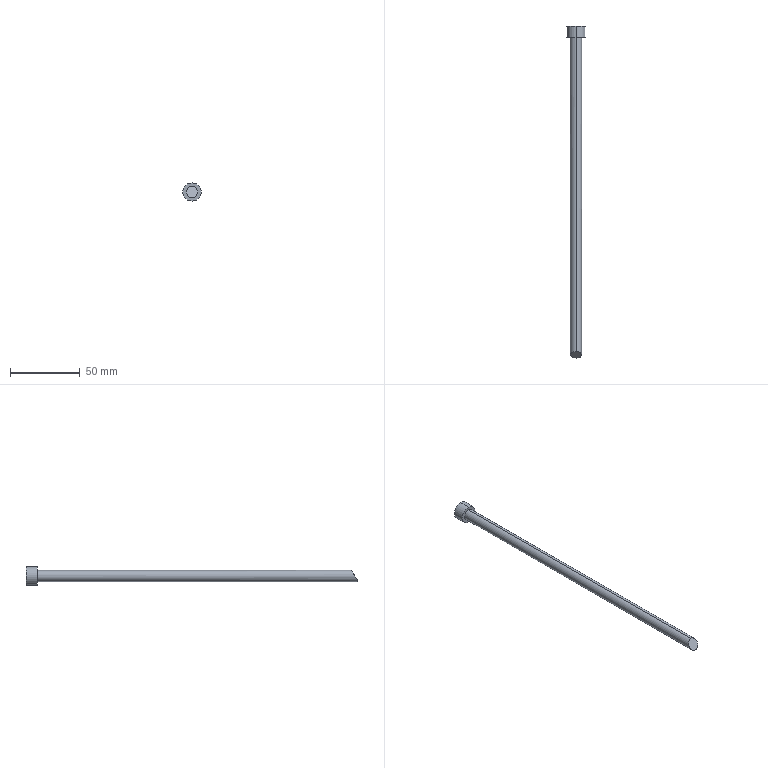Part | STEP file | 1 solid | 7 faces | box 13 x 237.193 x 13 mm | volume 12467 mm3 | cylinder 4 | plane 3 | commonest cylinder face diameters 8 x2 13 x2
STEP:
#1=CARTESIAN_POINT('',(0.,0.,0.));
#2=DIRECTION('',(0.,0.,1.));
#3=DIRECTION('',(1.,0.,0.));
#4=AXIS2_PLACEMENT_3D('',#1,#2,#3);
#5=CARTESIAN_POINT('',(-72.862,290.5,201.029));
#6=VERTEX_POINT('',#5);
#7=CARTESIAN_POINT('',(-72.862,290.5,214.029));
#8=VERTEX_POINT('',#7);
#9=CARTESIAN_POINT('',(-72.862,290.5,207.529));
#10=DIRECTION('',(0.,-1.,0.));
#11=DIRECTION('',(0.,0.,-1.));
#12=AXIS2_PLACEMENT_3D('',#9,#10,#11);
#13=CIRCLE('',#12,6.5);
#14=CARTESIAN_POINT('',(-72.862,290.5,207.529));
#15=DIRECTION('',(0.,-1.,0.));
#16=DIRECTION('',(0.,0.,-1.));
#17=AXIS2_PLACEMENT_3D('',#14,#15,#16);
#18=CYLINDRICAL_SURFACE('',#17,6.5);
#19=CARTESIAN_POINT('',(0.,0.));
#20=DIRECTION('',(1.,0.));
#21=VECTOR('',#20,1.);
#22=LINE('',#19,#21);
#23=(GEOMETRIC_REPRESENTATION_CONTEXT(2)PARAMETRIC_REPRESENTATION_CONTEXT()REPRESENTATION_CONTEXT('',''));
#24=DEFINITIONAL_REPRESENTATION('',(#22),#23);
#25=PCURVE('',#18,#24);
#26=CARTESIAN_POINT('',(-72.862,290.5,110.196));
#27=DIRECTION('',(0.,-1.,0.));
#28=DIRECTION('',(0.,0.,-1.));
#29=AXIS2_PLACEMENT_3D('',#26,#27,#28);
#30=PLANE('',#29);
#31=CARTESIAN_POINT('',(-97.333,-0.000000011));
#32=DIRECTION('',(1.,0.));
#33=AXIS2_PLACEMENT_2D('',#31,#32);
#34=CIRCLE('',#33,6.5);
#35=(GEOMETRIC_REPRESENTATION_CONTEXT(2)PARAMETRIC_REPRESENTATION_CONTEXT()REPRESENTATION_CONTEXT('',''));
#36=DEFINITIONAL_REPRESENTATION('',(#34),#35);
#37=PCURVE('',#30,#36);
#38=SURFACE_CURVE('',#13,(#25,#37),.PCURVE_S1.);
#39=EDGE_CURVE('',#6,#8,#38,.T.);
#40=ORIENTED_EDGE('',*,*,#39,.T.);
#41=CARTESIAN_POINT('',(-72.862,282.5,214.029));
#42=VERTEX_POINT('',#41);
#43=CARTESIAN_POINT('',(-72.862,290.5,214.029));
#44=DIRECTION('',(0.,-1.,0.));
#45=VECTOR('',#44,1.);
#46=LINE('',#43,#45);
#47=CARTESIAN_POINT('',(3.142,0.));
#48=DIRECTION('',(0.,1.));
#49=VECTOR('',#48,1.);
#50=LINE('',#47,#49);
#51=(GEOMETRIC_REPRESENTATION_CONTEXT(2)PARAMETRIC_REPRESENTATION_CONTEXT()REPRESENTATION_CONTEXT('',''));
#52=DEFINITIONAL_REPRESENTATION('',(#50),#51);
#53=PCURVE('',#18,#52);
#54=CARTESIAN_POINT('',(-72.862,290.5,207.529));
#55=DIRECTION('',(0.,-1.,0.));
#56=DIRECTION('',(0.,0.,-1.));
#57=AXIS2_PLACEMENT_3D('',#54,#55,#56);
#58=CYLINDRICAL_SURFACE('',#57,6.5);
#59=CARTESIAN_POINT('',(3.142,0.));
#60=DIRECTION('',(0.,1.));
#61=VECTOR('',#60,1.);
#62=LINE('',#59,#61);
#63=(GEOMETRIC_REPRESENTATION_CONTEXT(2)PARAMETRIC_REPRESENTATION_CONTEXT()REPRESENTATION_CONTEXT('',''));
#64=DEFINITIONAL_REPRESENTATION('',(#62),#63);
#65=PCURVE('',#58,#64);
#66=SURFACE_CURVE('',#46,(#53,#65),.PCURVE_S1.);
#67=EDGE_CURVE('',#8,#42,#66,.T.);
#68=ORIENTED_EDGE('',*,*,#67,.T.);
#69=CARTESIAN_POINT('',(-72.862,282.5,201.029));
#70=VERTEX_POINT('',#69);
#71=CARTESIAN_POINT('',(-72.862,282.5,207.529));
#72=DIRECTION('',(0.,1.,0.));
#73=DIRECTION('',(0.,0.,1.));
#74=AXIS2_PLACEMENT_3D('',#71,#72,#73);
#75=CIRCLE('',#74,6.5);
#76=CARTESIAN_POINT('',(3.142,8.));
#77=DIRECTION('',(-1.,0.));
#78=VECTOR('',#77,1.);
#79=LINE('',#76,#78);
#80=(GEOMETRIC_REPRESENTATION_CONTEXT(2)PARAMETRIC_REPRESENTATION_CONTEXT()REPRESENTATION_CONTEXT('',''));
#81=DEFINITIONAL_REPRESENTATION('',(#79),#80);
#82=PCURVE('',#18,#81);
#83=CARTESIAN_POINT('',(-72.862,282.5,207.529));
#84=DIRECTION('',(0.,-1.,0.));
#85=DIRECTION('',(0.,0.,-1.));
#86=AXIS2_PLACEMENT_3D('',#83,#84,#85);
#87=PLANE('',#86);
#88=CARTESIAN_POINT('',(-6.5,0.));
#89=CARTESIAN_POINT('',(-6.5,11.258));
#90=CARTESIAN_POINT('',(3.25,5.629));
#91=CARTESIAN_POINT('',(13.,0.));
#92=CARTESIAN_POINT('',(3.25,-5.629));
#93=CARTESIAN_POINT('',(-6.5,-11.258));
#94=CARTESIAN_POINT('',(-6.5,0.));
#95=(BOUNDED_CURVE()B_SPLINE_CURVE(2,(#88,#89,#90,#91,#92,#93,#94),.UNSPECIFIED.,.T.,.F.)B_SPLINE_CURVE_WITH_KNOTS((1,2,2,2,2,1),(-2.094,0.,2.094,4.189,6.283,8.378),.UNSPECIFIED.)CURVE()GEOMETRIC_REPRESENTATION_ITEM()RATIONAL_B_SPLINE_CURVE((1.,0.5,1.,0.5,1.,0.5,1.))REPRESENTATION_ITEM(''));
#96=(GEOMETRIC_REPRESENTATION_CONTEXT(2)PARAMETRIC_REPRESENTATION_CONTEXT()REPRESENTATION_CONTEXT('',''));
#97=DEFINITIONAL_REPRESENTATION('',(#95),#96);
#98=PCURVE('',#87,#97);
#99=SURFACE_CURVE('',#75,(#82,#98),.PCURVE_S1.);
#100=EDGE_CURVE('',#42,#70,#99,.T.);
#101=ORIENTED_EDGE('',*,*,#100,.T.);
#102=CARTESIAN_POINT('',(-72.862,290.5,201.029));
#103=DIRECTION('',(0.,-1.,0.));
#104=VECTOR('',#103,1.);
#105=LINE('',#102,#104);
#106=CARTESIAN_POINT('',(0.,0.));
#107=DIRECTION('',(0.,1.));
#108=VECTOR('',#107,1.);
#109=LINE('',#106,#108);
#110=(GEOMETRIC_REPRESENTATION_CONTEXT(2)PARAMETRIC_REPRESENTATION_CONTEXT()REPRESENTATION_CONTEXT('',''));
#111=DEFINITIONAL_REPRESENTATION('',(#109),#110);
#112=PCURVE('',#18,#111);
#113=CARTESIAN_POINT('',(6.283,0.));
#114=DIRECTION('',(0.,1.));
#115=VECTOR('',#114,1.);
#116=LINE('',#113,#115);
#117=(GEOMETRIC_REPRESENTATION_CONTEXT(2)PARAMETRIC_REPRESENTATION_CONTEXT()REPRESENTATION_CONTEXT('',''));
#118=DEFINITIONAL_REPRESENTATION('',(#116),#117);
#119=PCURVE('',#58,#118);
#120=SURFACE_CURVE('',#105,(#112,#119),.PCURVE_S1.);
#121=EDGE_CURVE('',#6,#70,#120,.T.);
#122=ORIENTED_EDGE('',*,*,#121,.F.);
#123=EDGE_LOOP('',(#40,#68,#101,#122));
#124=FACE_BOUND('',#123,.T.);
#125=ADVANCED_FACE('',(#124),#18,.T.);
#126=CARTESIAN_POINT('',(-72.862,282.5,211.529));
#127=VERTEX_POINT('',#126);
#128=CARTESIAN_POINT('',(-72.862,282.5,203.529));
#129=VERTEX_POINT('',#128);
#130=CARTESIAN_POINT('',(-72.862,282.5,207.529));
#131=DIRECTION('',(0.,1.,0.));
#132=DIRECTION('',(0.,0.,-1.));
#133=AXIS2_PLACEMENT_3D('',#130,#131,#132);
#134=CIRCLE('',#133,4.);
#135=CARTESIAN_POINT('',(-72.862,220.5,207.529));
#136=DIRECTION('',(0.,-1.,0.));
#137=DIRECTION('',(0.,0.,-1.));
#138=AXIS2_PLACEMENT_3D('',#135,#136,#137);
#139=CYLINDRICAL_SURFACE('',#138,4.);
#140=CARTESIAN_POINT('',(6.283,-62.));
#141=DIRECTION('',(-1.,0.));
#142=VECTOR('',#141,1.);
#143=LINE('',#140,#142);
#144=(GEOMETRIC_REPRESENTATION_CONTEXT(2)PARAMETRIC_REPRESENTATION_CONTEXT()REPRESENTATION_CONTEXT('',''));
#145=DEFINITIONAL_REPRESENTATION('',(#143),#144);
#146=PCURVE('',#139,#145);
#147=CARTESIAN_POINT('',(4.,0.));
#148=CARTESIAN_POINT('',(4.,-6.928));
#149=CARTESIAN_POINT('',(-2.,-3.464));
#150=CARTESIAN_POINT('',(-8.,0.));
#151=CARTESIAN_POINT('',(-2.,3.464));
#152=CARTESIAN_POINT('',(4.,6.928));
#153=CARTESIAN_POINT('',(4.,0.));
#154=(BOUNDED_CURVE()B_SPLINE_CURVE(2,(#147,#148,#149,#150,#151,#152,#153),.UNSPECIFIED.,.T.,.F.)B_SPLINE_CURVE_WITH_KNOTS((1,2,2,2,2,1),(-2.094,0.,2.094,4.189,6.283,8.378),.UNSPECIFIED.)CURVE()GEOMETRIC_REPRESENTATION_ITEM()RATIONAL_B_SPLINE_CURVE((1.,0.5,1.,0.5,1.,0.5,1.))REPRESENTATION_ITEM(''));
#155=(GEOMETRIC_REPRESENTATION_CONTEXT(2)PARAMETRIC_REPRESENTATION_CONTEXT()REPRESENTATION_CONTEXT('',''));
#156=DEFINITIONAL_REPRESENTATION('',(#154),#155);
#157=PCURVE('',#87,#156);
#158=SURFACE_CURVE('',#134,(#146,#157),.PCURVE_S1.);
#159=EDGE_CURVE('',#127,#129,#158,.T.);
#160=ORIENTED_EDGE('',*,*,#159,.F.);
#161=CARTESIAN_POINT('',(-72.862,57.925,211.529));
#162=VERTEX_POINT('',#161);
#163=CARTESIAN_POINT('',(-72.862,220.5,211.529));
#164=DIRECTION('',(0.,-1.,0.));
#165=VECTOR('',#164,1.);
#166=LINE('',#163,#165);
#167=CARTESIAN_POINT('',(3.142,0.));
#168=DIRECTION('',(0.,1.));
#169=VECTOR('',#168,1.);
#170=LINE('',#167,#169);
#171=(GEOMETRIC_REPRESENTATION_CONTEXT(2)PARAMETRIC_REPRESENTATION_CONTEXT()REPRESENTATION_CONTEXT('',''));
#172=DEFINITIONAL_REPRESENTATION('',(#170),#171);
#173=PCURVE('',#139,#172);
#174=CARTESIAN_POINT('',(-72.862,220.5,207.529));
#175=DIRECTION('',(0.,-1.,0.));
#176=DIRECTION('',(0.,0.,-1.));
#177=AXIS2_PLACEMENT_3D('',#174,#175,#176);
#178=CYLINDRICAL_SURFACE('',#177,4.);
#179=CARTESIAN_POINT('',(3.142,0.));
#180=DIRECTION('',(0.,1.));
#181=VECTOR('',#180,1.);
#182=LINE('',#179,#181);
#183=(GEOMETRIC_REPRESENTATION_CONTEXT(2)PARAMETRIC_REPRESENTATION_CONTEXT()REPRESENTATION_CONTEXT('',''));
#184=DEFINITIONAL_REPRESENTATION('',(#182),#183);
#185=PCURVE('',#178,#184);
#186=SURFACE_CURVE('',#166,(#173,#185),.PCURVE_S1.);
#187=EDGE_CURVE('',#127,#162,#186,.T.);
#188=ORIENTED_EDGE('',*,*,#187,.T.);
#189=CARTESIAN_POINT('',(-72.862,53.307,203.529));
#190=VERTEX_POINT('',#189);
#191=CARTESIAN_POINT('',(-72.862,53.307,203.529));
#192=CARTESIAN_POINT('',(-64.862,53.307,203.529));
#193=CARTESIAN_POINT('',(-64.862,57.925,211.529));
#194=CARTESIAN_POINT('',(-72.862,57.925,211.529));
#195=(BOUNDED_CURVE()B_SPLINE_CURVE(3,(#191,#192,#193,#194),.UNSPECIFIED.,.F.,.F.)B_SPLINE_CURVE_WITH_KNOTS((4,4),(0.,3.142),.PIECEWISE_BEZIER_KNOTS.)CURVE()GEOMETRIC_REPRESENTATION_ITEM()RATIONAL_B_SPLINE_CURVE((1.,0.3333,0.3333,1.))REPRESENTATION_ITEM(''));
#196=CARTESIAN_POINT('',(0.,167.193));
#197=CARTESIAN_POINT('',(0.0303,167.193));
#198=CARTESIAN_POINT('',(0.09367,167.187));
#199=CARTESIAN_POINT('',(0.1977,167.153));
#200=CARTESIAN_POINT('',(0.3115,167.087));
#201=CARTESIAN_POINT('',(0.4356,166.984));
#202=CARTESIAN_POINT('',(0.5703,166.834));
#203=CARTESIAN_POINT('',(0.7158,166.633));
#204=CARTESIAN_POINT('',(0.8717,166.377));
#205=CARTESIAN_POINT('',(1.037,166.065));
#206=CARTESIAN_POINT('',(1.21,165.703));
#207=CARTESIAN_POINT('',(1.389,165.304));
#208=CARTESIAN_POINT('',(1.571,164.884));
#209=CARTESIAN_POINT('',(1.753,164.464));
#210=CARTESIAN_POINT('',(1.931,164.065));
#211=CARTESIAN_POINT('',(2.105,163.703));
#212=CARTESIAN_POINT('',(2.27,163.391));
#213=CARTESIAN_POINT('',(2.426,163.135));
#214=CARTESIAN_POINT('',(2.571,162.934));
#215=CARTESIAN_POINT('',(2.706,162.784));
#216=CARTESIAN_POINT('',(2.83,162.681));
#217=CARTESIAN_POINT('',(2.944,162.615));
#218=CARTESIAN_POINT('',(3.048,162.581));
#219=CARTESIAN_POINT('',(3.111,162.575));
#220=CARTESIAN_POINT('',(3.142,162.575));
#221=B_SPLINE_CURVE_WITH_KNOTS('',3,(#196,#197,#198,#199,#200,#201,#202,#203,#204,#205,#206,#207,#208,#209,#210,#211,#212,#213,#214,#215,#216,#217,#218,#219,#220),.UNSPECIFIED.,.F.,.F.,(4,1,1,1,1,1,1,1,1,1,1,1,1,1,1,1,1,1,1,1,1,1,4),(0.,0.1428,0.2856,0.4284,0.5712,0.714,0.8568,0.9996,1.142,1.285,1.428,1.571,1.714,1.856,1.999,2.142,2.285,2.428,2.57,2.713,2.856,2.999,3.142),.QUASI_UNIFORM_KNOTS.);
#222=(GEOMETRIC_REPRESENTATION_CONTEXT(2)PARAMETRIC_REPRESENTATION_CONTEXT()REPRESENTATION_CONTEXT('',''));
#223=DEFINITIONAL_REPRESENTATION('',(#221),#222);
#224=PCURVE('',#139,#223);
#225=CARTESIAN_POINT('',(-98.49,38.356,177.634));
#226=DIRECTION('',(0.,0.866,-0.5));
#227=DIRECTION('',(0.,0.5,0.866));
#228=AXIS2_PLACEMENT_3D('',#225,#226,#227);
#229=PLANE('',#228);
#230=CARTESIAN_POINT('',(29.901,25.628));
#231=CARTESIAN_POINT('',(29.901,33.627));
#232=CARTESIAN_POINT('',(39.139,33.627));
#233=CARTESIAN_POINT('',(39.139,25.628));
#234=(BOUNDED_CURVE()B_SPLINE_CURVE(3,(#230,#231,#232,#233),.UNSPECIFIED.,.F.,.F.)B_SPLINE_CURVE_WITH_KNOTS((4,4),(0.,3.142),.PIECEWISE_BEZIER_KNOTS.)CURVE()GEOMETRIC_REPRESENTATION_ITEM()RATIONAL_B_SPLINE_CURVE((1.,0.3333,0.3333,1.))REPRESENTATION_ITEM(''));
#235=(GEOMETRIC_REPRESENTATION_CONTEXT(2)PARAMETRIC_REPRESENTATION_CONTEXT()REPRESENTATION_CONTEXT('',''));
#236=DEFINITIONAL_REPRESENTATION('',(#234),#235);
#237=PCURVE('',#229,#236);
#238=SURFACE_CURVE('',#195,(#224,#237),.PCURVE_S1.);
#239=EDGE_CURVE('',#190,#162,#238,.T.);
#240=ORIENTED_EDGE('',*,*,#239,.F.);
#241=CARTESIAN_POINT('',(-72.862,220.5,203.529));
#242=DIRECTION('',(0.,-1.,0.));
#243=VECTOR('',#242,1.);
#244=LINE('',#241,#243);
#245=CARTESIAN_POINT('',(0.,0.));
#246=DIRECTION('',(0.,1.));
#247=VECTOR('',#246,1.);
#248=LINE('',#245,#247);
#249=(GEOMETRIC_REPRESENTATION_CONTEXT(2)PARAMETRIC_REPRESENTATION_CONTEXT()REPRESENTATION_CONTEXT('',''));
#250=DEFINITIONAL_REPRESENTATION('',(#248),#249);
#251=PCURVE('',#139,#250);
#252=CARTESIAN_POINT('',(6.283,0.));
#253=DIRECTION('',(0.,1.));
#254=VECTOR('',#253,1.);
#255=LINE('',#252,#254);
#256=(GEOMETRIC_REPRESENTATION_CONTEXT(2)PARAMETRIC_REPRESENTATION_CONTEXT()REPRESENTATION_CONTEXT('',''));
#257=DEFINITIONAL_REPRESENTATION('',(#255),#256);
#258=PCURVE('',#178,#257);
#259=SURFACE_CURVE('',#244,(#251,#258),.PCURVE_S1.);
#260=EDGE_CURVE('',#129,#190,#259,.T.);
#261=ORIENTED_EDGE('',*,*,#260,.F.);
#262=EDGE_LOOP('',(#160,#188,#240,#261));
#263=FACE_BOUND('',#262,.T.);
#264=ADVANCED_FACE('',(#263),#139,.T.);
#265=ORIENTED_EDGE('',*,*,#239,.T.);
#266=CARTESIAN_POINT('',(-72.862,57.925,211.529));
#267=CARTESIAN_POINT('',(-80.862,57.925,211.529));
#268=CARTESIAN_POINT('',(-80.862,53.307,203.529));
#269=CARTESIAN_POINT('',(-72.862,53.307,203.529));
#270=(BOUNDED_CURVE()B_SPLINE_CURVE(3,(#266,#267,#268,#269),.UNSPECIFIED.,.F.,.F.)B_SPLINE_CURVE_WITH_KNOTS((4,4),(3.142,6.283),.PIECEWISE_BEZIER_KNOTS.)CURVE()GEOMETRIC_REPRESENTATION_ITEM()RATIONAL_B_SPLINE_CURVE((1.,0.3333,0.3333,1.))REPRESENTATION_ITEM(''));
#271=CARTESIAN_POINT('',(39.139,25.628));
#272=CARTESIAN_POINT('',(39.139,17.628));
#273=CARTESIAN_POINT('',(29.901,17.628));
#274=CARTESIAN_POINT('',(29.901,25.628));
#275=(BOUNDED_CURVE()B_SPLINE_CURVE(3,(#271,#272,#273,#274),.UNSPECIFIED.,.F.,.F.)B_SPLINE_CURVE_WITH_KNOTS((4,4),(3.142,6.283),.PIECEWISE_BEZIER_KNOTS.)CURVE()GEOMETRIC_REPRESENTATION_ITEM()RATIONAL_B_SPLINE_CURVE((1.,0.3333,0.3333,1.))REPRESENTATION_ITEM(''));
#276=(GEOMETRIC_REPRESENTATION_CONTEXT(2)PARAMETRIC_REPRESENTATION_CONTEXT()REPRESENTATION_CONTEXT('',''));
#277=DEFINITIONAL_REPRESENTATION('',(#275),#276);
#278=PCURVE('',#229,#277);
#279=CARTESIAN_POINT('',(3.142,162.575));
#280=CARTESIAN_POINT('',(3.172,162.575));
#281=CARTESIAN_POINT('',(3.235,162.581));
#282=CARTESIAN_POINT('',(3.339,162.615));
#283=CARTESIAN_POINT('',(3.453,162.681));
#284=CARTESIAN_POINT('',(3.577,162.784));
#285=CARTESIAN_POINT('',(3.712,162.934));
#286=CARTESIAN_POINT('',(3.857,163.135));
#287=CARTESIAN_POINT('',(4.013,163.391));
#288=CARTESIAN_POINT('',(4.179,163.703));
#289=CARTESIAN_POINT('',(4.352,164.065));
#290=CARTESIAN_POINT('',(4.531,164.464));
#291=CARTESIAN_POINT('',(4.712,164.884));
#292=CARTESIAN_POINT('',(4.894,165.304));
#293=CARTESIAN_POINT('',(5.073,165.703));
#294=CARTESIAN_POINT('',(5.246,166.065));
#295=CARTESIAN_POINT('',(5.412,166.377));
#296=CARTESIAN_POINT('',(5.567,166.633));
#297=CARTESIAN_POINT('',(5.713,166.834));
#298=CARTESIAN_POINT('',(5.848,166.984));
#299=CARTESIAN_POINT('',(5.972,167.087));
#300=CARTESIAN_POINT('',(6.085,167.153));
#301=CARTESIAN_POINT('',(6.19,167.187));
#302=CARTESIAN_POINT('',(6.253,167.193));
#303=CARTESIAN_POINT('',(6.283,167.193));
#304=B_SPLINE_CURVE_WITH_KNOTS('',3,(#279,#280,#281,#282,#283,#284,#285,#286,#287,#288,#289,#290,#291,#292,#293,#294,#295,#296,#297,#298,#299,#300,#301,#302,#303),.UNSPECIFIED.,.F.,.F.,(4,1,1,1,1,1,1,1,1,1,1,1,1,1,1,1,1,1,1,1,1,1,4),(3.142,3.284,3.427,3.57,3.713,3.856,3.998,4.141,4.284,4.427,4.57,4.712,4.855,4.998,5.141,5.284,5.426,5.569,5.712,5.855,5.998,6.14,6.283),.QUASI_UNIFORM_KNOTS.);
#305=(GEOMETRIC_REPRESENTATION_CONTEXT(2)PARAMETRIC_REPRESENTATION_CONTEXT()REPRESENTATION_CONTEXT('',''));
#306=DEFINITIONAL_REPRESENTATION('',(#304),#305);
#307=PCURVE('',#178,#306);
#308=SURFACE_CURVE('',#270,(#278,#307),.PCURVE_S1.);
#309=EDGE_CURVE('',#162,#190,#308,.T.);
#310=ORIENTED_EDGE('',*,*,#309,.T.);
#311=EDGE_LOOP('',(#265,#310));
#312=FACE_BOUND('',#311,.T.);
#313=ADVANCED_FACE('',(#312),#229,.F.);
#314=ORIENTED_EDGE('',*,*,#187,.F.);
#315=CARTESIAN_POINT('',(-72.862,282.5,207.529));
#316=DIRECTION('',(0.,1.,0.));
#317=DIRECTION('',(0.,0.,-1.));
#318=AXIS2_PLACEMENT_3D('',#315,#316,#317);
#319=CIRCLE('',#318,4.);
#320=CARTESIAN_POINT('',(6.283,-62.));
#321=DIRECTION('',(-1.,0.));
#322=VECTOR('',#321,1.);
#323=LINE('',#320,#322);
#324=(GEOMETRIC_REPRESENTATION_CONTEXT(2)PARAMETRIC_REPRESENTATION_CONTEXT()REPRESENTATION_CONTEXT('',''));
#325=DEFINITIONAL_REPRESENTATION('',(#323),#324);
#326=PCURVE('',#178,#325);
#327=CARTESIAN_POINT('',(4.,0.));
#328=CARTESIAN_POINT('',(4.,-6.928));
#329=CARTESIAN_POINT('',(-2.,-3.464));
#330=CARTESIAN_POINT('',(-8.,0.));
#331=CARTESIAN_POINT('',(-2.,3.464));
#332=CARTESIAN_POINT('',(4.,6.928));
#333=CARTESIAN_POINT('',(4.,0.));
#334=(BOUNDED_CURVE()B_SPLINE_CURVE(2,(#327,#328,#329,#330,#331,#332,#333),.UNSPECIFIED.,.T.,.F.)B_SPLINE_CURVE_WITH_KNOTS((1,2,2,2,2,1),(-2.094,0.,2.094,4.189,6.283,8.378),.UNSPECIFIED.)CURVE()GEOMETRIC_REPRESENTATION_ITEM()RATIONAL_B_SPLINE_CURVE((1.,0.5,1.,0.5,1.,0.5,1.))REPRESENTATION_ITEM(''));
#335=(GEOMETRIC_REPRESENTATION_CONTEXT(2)PARAMETRIC_REPRESENTATION_CONTEXT()REPRESENTATION_CONTEXT('',''));
#336=DEFINITIONAL_REPRESENTATION('',(#334),#335);
#337=PCURVE('',#87,#336);
#338=SURFACE_CURVE('',#319,(#326,#337),.PCURVE_S1.);
#339=EDGE_CURVE('',#129,#127,#338,.T.);
#340=ORIENTED_EDGE('',*,*,#339,.F.);
#341=ORIENTED_EDGE('',*,*,#260,.T.);
#342=ORIENTED_EDGE('',*,*,#309,.F.);
#343=EDGE_LOOP('',(#314,#340,#341,#342));
#344=FACE_BOUND('',#343,.T.);
#345=ADVANCED_FACE('',(#344),#178,.T.);
#346=ORIENTED_EDGE('',*,*,#339,.T.);
#347=ORIENTED_EDGE('',*,*,#159,.T.);
#348=EDGE_LOOP('',(#346,#347));
#349=FACE_BOUND('',#348,.T.);
#350=CARTESIAN_POINT('',(-72.862,282.5,207.529));
#351=DIRECTION('',(0.,1.,0.));
#352=DIRECTION('',(0.,0.,1.));
#353=AXIS2_PLACEMENT_3D('',#350,#351,#352);
#354=CIRCLE('',#353,6.5);
#355=CARTESIAN_POINT('',(-6.5,0.));
#356=CARTESIAN_POINT('',(-6.5,11.258));
#357=CARTESIAN_POINT('',(3.25,5.629));
#358=CARTESIAN_POINT('',(13.,0.));
#359=CARTESIAN_POINT('',(3.25,-5.629));
#360=CARTESIAN_POINT('',(-6.5,-11.258));
#361=CARTESIAN_POINT('',(-6.5,0.));
#362=(BOUNDED_CURVE()B_SPLINE_CURVE(2,(#355,#356,#357,#358,#359,#360,#361),.UNSPECIFIED.,.T.,.F.)B_SPLINE_CURVE_WITH_KNOTS((1,2,2,2,2,1),(-2.094,0.,2.094,4.189,6.283,8.378),.UNSPECIFIED.)CURVE()GEOMETRIC_REPRESENTATION_ITEM()RATIONAL_B_SPLINE_CURVE((1.,0.5,1.,0.5,1.,0.5,1.))REPRESENTATION_ITEM(''));
#363=(GEOMETRIC_REPRESENTATION_CONTEXT(2)PARAMETRIC_REPRESENTATION_CONTEXT()REPRESENTATION_CONTEXT('',''));
#364=DEFINITIONAL_REPRESENTATION('',(#362),#363);
#365=PCURVE('',#87,#364);
#366=CARTESIAN_POINT('',(9.425,8.));
#367=DIRECTION('',(-1.,0.));
#368=VECTOR('',#367,1.);
#369=LINE('',#366,#368);
#370=(GEOMETRIC_REPRESENTATION_CONTEXT(2)PARAMETRIC_REPRESENTATION_CONTEXT()REPRESENTATION_CONTEXT('',''));
#371=DEFINITIONAL_REPRESENTATION('',(#369),#370);
#372=PCURVE('',#58,#371);
#373=SURFACE_CURVE('',#354,(#365,#372),.PCURVE_S1.);
#374=EDGE_CURVE('',#70,#42,#373,.T.);
#375=ORIENTED_EDGE('',*,*,#374,.F.);
#376=ORIENTED_EDGE('',*,*,#100,.F.);
#377=EDGE_LOOP('',(#375,#376));
#378=FACE_BOUND('',#377,.T.);
#379=ADVANCED_FACE('',(#349,#378),#87,.T.);
#380=ORIENTED_EDGE('',*,*,#67,.F.);
#381=CARTESIAN_POINT('',(-72.862,290.5,207.529));
#382=DIRECTION('',(0.,-1.,0.));
#383=DIRECTION('',(0.,0.,-1.));
#384=AXIS2_PLACEMENT_3D('',#381,#382,#383);
#385=CIRCLE('',#384,6.5);
#386=CARTESIAN_POINT('',(0.,0.));
#387=DIRECTION('',(1.,0.));
#388=VECTOR('',#387,1.);
#389=LINE('',#386,#388);
#390=(GEOMETRIC_REPRESENTATION_CONTEXT(2)PARAMETRIC_REPRESENTATION_CONTEXT()REPRESENTATION_CONTEXT('',''));
#391=DEFINITIONAL_REPRESENTATION('',(#389),#390);
#392=PCURVE('',#58,#391);
#393=CARTESIAN_POINT('',(-97.333,-0.000000011));
#394=DIRECTION('',(1.,0.));
#395=AXIS2_PLACEMENT_2D('',#393,#394);
#396=CIRCLE('',#395,6.5);
#397=(GEOMETRIC_REPRESENTATION_CONTEXT(2)PARAMETRIC_REPRESENTATION_CONTEXT()REPRESENTATION_CONTEXT('',''));
#398=DEFINITIONAL_REPRESENTATION('',(#396),#397);
#399=PCURVE('',#30,#398);
#400=SURFACE_CURVE('',#385,(#392,#399),.PCURVE_S1.);
#401=EDGE_CURVE('',#8,#6,#400,.T.);
#402=ORIENTED_EDGE('',*,*,#401,.T.);
#403=ORIENTED_EDGE('',*,*,#121,.T.);
#404=ORIENTED_EDGE('',*,*,#374,.T.);
#405=EDGE_LOOP('',(#380,#402,#403,#404));
#406=FACE_BOUND('',#405,.T.);
#407=ADVANCED_FACE('',(#406),#58,.T.);
#408=ORIENTED_EDGE('',*,*,#39,.F.);
#409=ORIENTED_EDGE('',*,*,#401,.F.);
#410=EDGE_LOOP('',(#408,#409));
#411=FACE_BOUND('',#410,.T.);
#412=ADVANCED_FACE('',(#411),#30,.F.);
#413=CLOSED_SHELL('',(#125,#264,#313,#345,#379,#407,#412));
#414=MANIFOLD_SOLID_BREP('',#413);
#415=(LENGTH_UNIT()NAMED_UNIT(*)SI_UNIT(.MILLI.,.METRE.));
#416=UNCERTAINTY_MEASURE_WITH_UNIT(LENGTH_MEASURE(0.0000001),#415,'','');
#417=(NAMED_UNIT(*)PLANE_ANGLE_UNIT()SI_UNIT($,.RADIAN.));
#418=(NAMED_UNIT(*)SI_UNIT($,.STERADIAN.)SOLID_ANGLE_UNIT());
#419=(GEOMETRIC_REPRESENTATION_CONTEXT(3)GLOBAL_UNCERTAINTY_ASSIGNED_CONTEXT((#416))GLOBAL_UNIT_ASSIGNED_CONTEXT((#415,#417,#418))REPRESENTATION_CONTEXT('',''));
#420=ADVANCED_BREP_SHAPE_REPRESENTATION('',(#4,#414),#419);